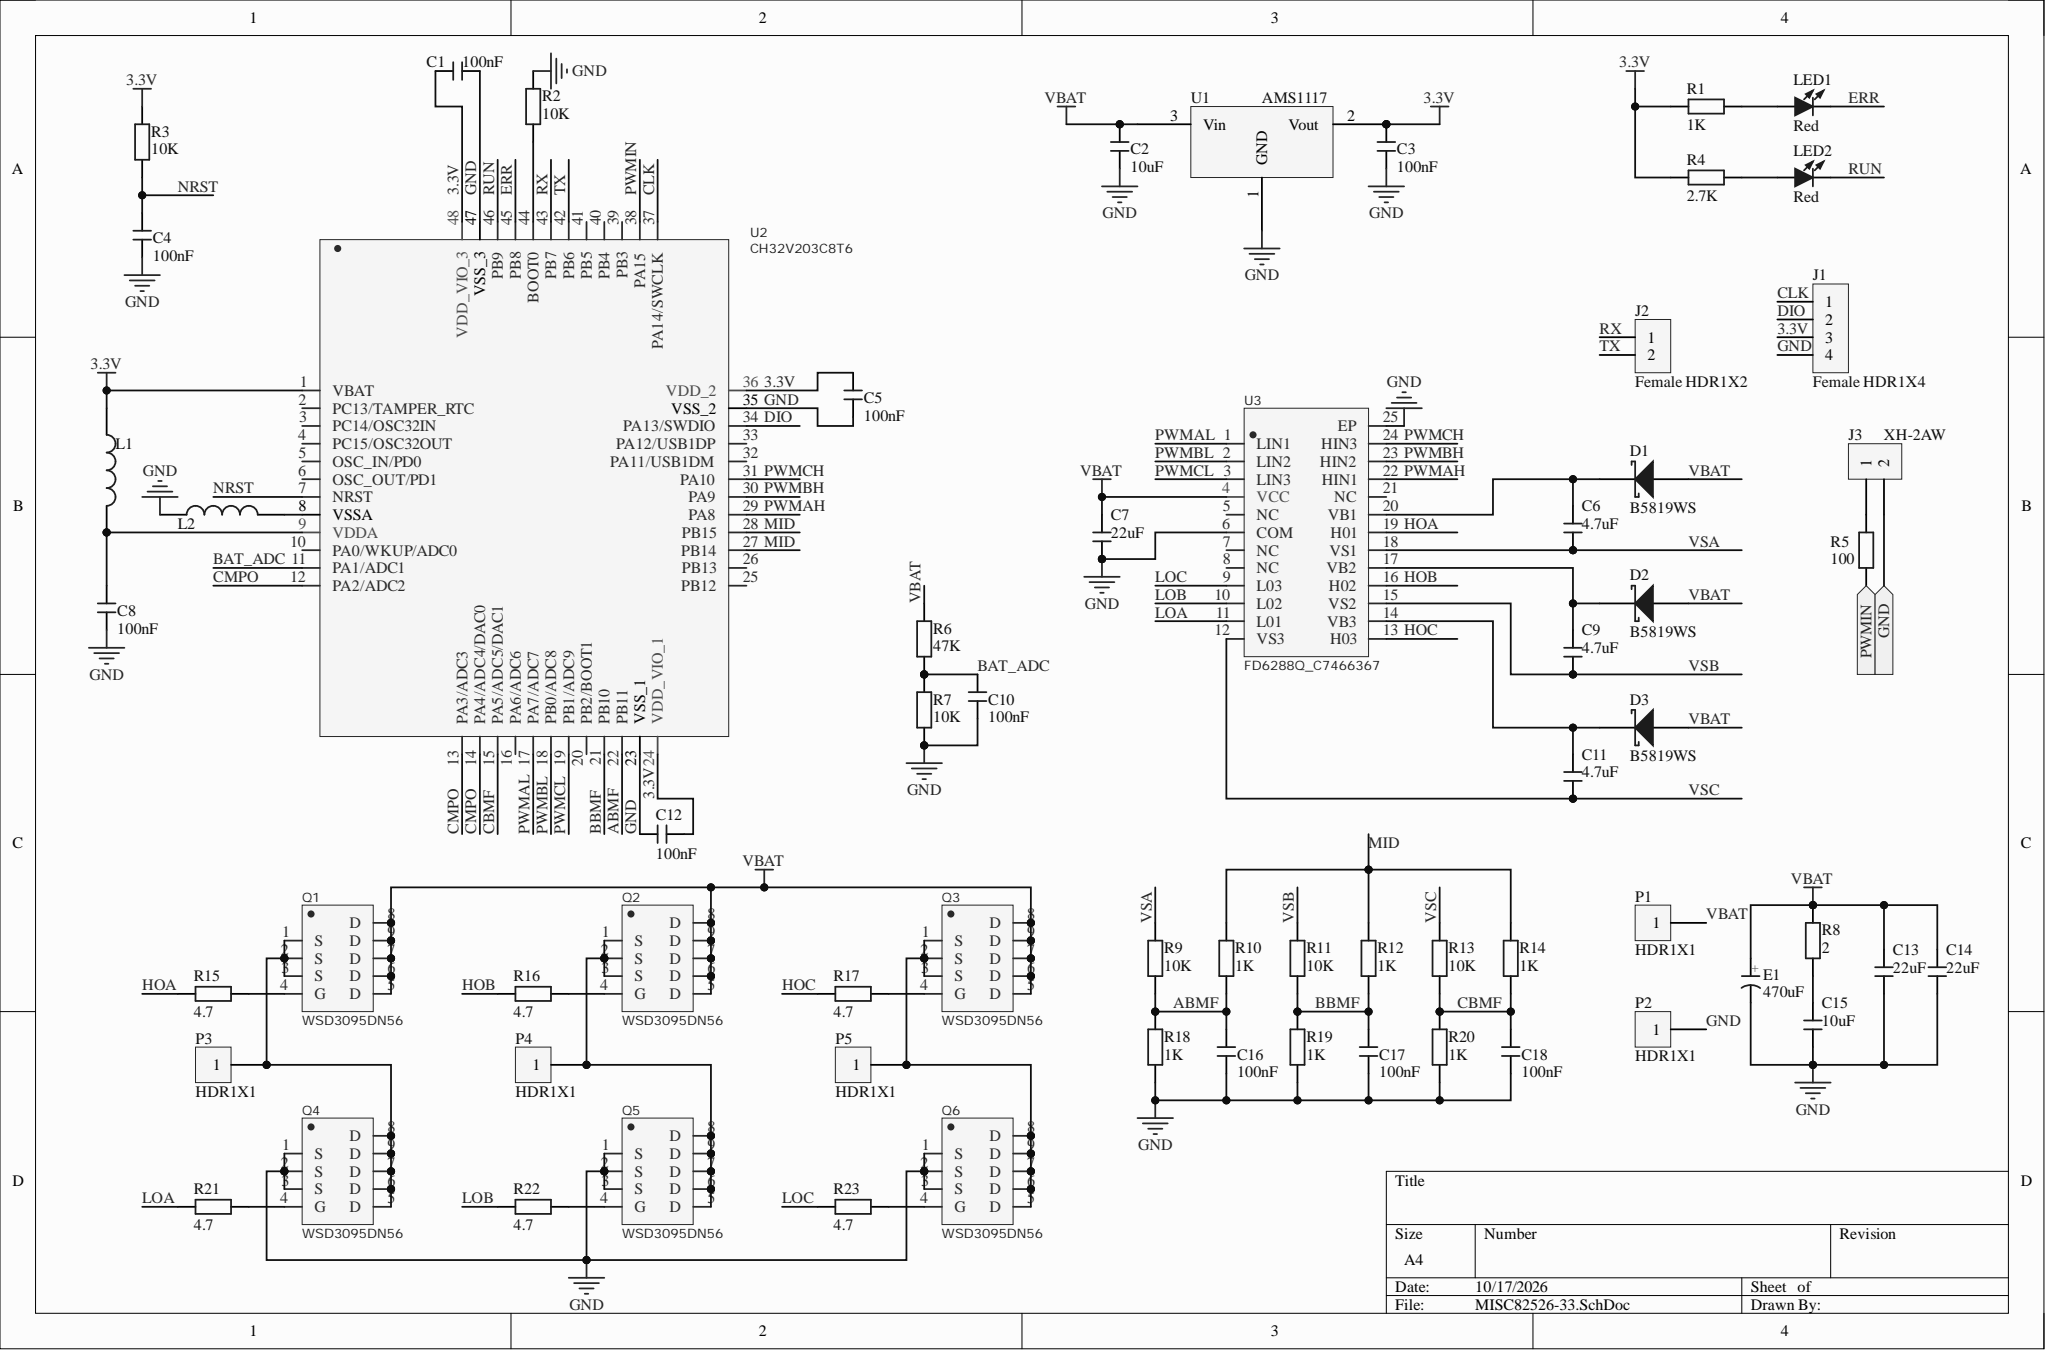Circuit board | Altium Designer | 66 parts | 50 nets
Bill of materials:
Comment,Description,Designator,Footprint,LibRef,Quantity
"100nF","SMD capacitor","C1, C3, C4, C5, C8, C10, C12, C16, C17, C18","C 0603_L","C","10"
"10uF","SMD capacitor","C2","C 0603_L","C","1"
"4.7uF","SMD capacitor","C6, C9, C11","C 0805_L","C","3"
"22uF","SMD capacitor","C7, C13, C14","C 0805_L","C","3"
"10uF","SMD capacitor","C15","C 0805_L","C","1"
"B5819WS","Schottky diode","D1, D2, D3","SOD-323","1N5819","3"
"470uF","SMD electrolytic capacitor","E1","CM A(3*5.4)","CE_SMD","1"
"Female HDR1X4","","J1","Fe-HDR1X4/2.54-S","Female HDR1X4","1"
"Female HDR1X2","","J2","Fe-HDR1X2/2.54-S","Female HDR1X2","1"
"XH-2AW","","J3","Fe-HDR1X2/2.54-S","Female HDR1X2","1"
"10uH","Low-power SMD inductor","L1, L2","L 0805","L","2"
"Red","SMD LED","LED1, LED2","LED 0805G","LED-SMD","2"
"HDR1X1","","P1, P2, P3, P4, P5","HDR1X1","HDR1X1","5"
"WSD3095DN56","","Q1, Q2, Q3, Q4, Q5, Q6","PDFN-8_L5.2-W5.9-P1.27-LS6.2-BL","WSD3095DN56","6"
"1K","SMD resistor","R1, R10, R12, R14, R18, R19, R20","R 0603_L","R","7"
"10K","SMD resistor","R2, R3, R7, R9, R11, R13","R 0603_L","R","6"
"2.7K","SMD resistor","R4","R 0603_L","R","1"
"100","SMD resistor","R5","R 0603_L","R","1"
"47K","SMD resistor","R6","R 0603_L","R","1"
"2","SMD resistor","R8","R 0603_L","R","1"
"4.7","SMD resistor","R15, R16, R17, R21, R22, R23","R 0603_L","R","6"
"AMS1117","Three-terminal voltage regulator","U1","SOT223","AMS1117","1"
"CH32V203C8T6","","U2","LQFP-48_L7.0-W7.0-P0.50-LS9.0-BL","CH32V203C8T6","1"
"FD6288Q_C7466367","","U3","QFN-24_L4.0-W4.0-P0.50-BL-EP2.7","FD6288Q_C7466367","1"
Netlist (Protel format):
[
C1
C 0603_L
100nF



]
[
C2
C 0603_L
10uF



]
[
C3
C 0603_L
100nF



]
[
C4
C 0603_L
100nF



]
[
C5
C 0603_L
100nF



]
[
C6
C 0805_L
4.7uF



]
[
C7
C 0805_L
22uF



]
[
C8
C 0603_L
100nF



]
[
C9
C 0805_L
4.7uF



]
[
C10
C 0603_L
100nF



]
[
C11
C 0805_L
4.7uF



]
[
C12
C 0603_L
100nF



]
[
C13
C 0805_L
22uF



]
[
C14
C 0805_L
22uF



]
[
C15
C 0805_L
10uF



]
[
C16
C 0603_L
100nF



]
[
C17
C 0603_L
100nF



]
[
C18
C 0603_L
100nF



]
[
D1
SOD-323
B5819WS



]
[
D2
SOD-323
B5819WS



]
[
D3
SOD-323
B5819WS



]
[
E1
CM A(3*5.4)
470uF



]
[
J1
Fe-HDR1X4/2.54-S
Female HDR1X4



]
[
J2
Fe-HDR1X2/2.54-S
Female HDR1X2



]
[
J3
Fe-HDR1X2/2.54-S
XH-2AW



]
[
L1
L 0805
10uH



]
[
L2
L 0805
10uH



]
[
LED1
LED 0805G
Red



]
[
LED2
LED 0805G
Red



]
[
P1
HDR1X1
HDR1X1



]
[
P2
HDR1X1
HDR1X1



]
[
P3
HDR1X1
HDR1X1



]
[
P4
HDR1X1
HDR1X1



]
[
P5
HDR1X1
HDR1X1



]
[
Q1
PDFN-8_L5.2-W5.9-P1.27-LS6.2-BL
WSD3095DN56



]
[
Q2
PDFN-8_L5.2-W5.9-P1.27-LS6.2-BL
WSD3095DN56



]
[
Q3
PDFN-8_L5.2-W5.9-P1.27-LS6.2-BL
WSD3095DN56



]
[
Q4
PDFN-8_L5.2-W5.9-P1.27-LS6.2-BL
WSD3095DN56



]
[
Q5
PDFN-8_L5.2-W5.9-P1.27-LS6.2-BL
WSD3095DN56



]
[
Q6
PDFN-8_L5.2-W5.9-P1.27-LS6.2-BL
WSD3095DN56



]
[
R1
R 0603_L
1K



]
[
R2
R 0603_L
10K



]
[
R3
R 0603_L
10K



]
[
R4
R 0603_L
2.7K



]
[
R5
R 0603_L
100



]
[
R6
R 0603_L
47K



]
[
R7
R 0603_L
10K



]
[
R8
R 0603_L
2



]
[
R9
R 0603_L
10K



]
[
R10
R 0603_L
1K



]
[
R11
R 0603_L
10K



]
[
R12
R 0603_L
1K



]
[
R13
R 0603_L
10K



]
[
R14
R 0603_L
1K



]
[
R15
R 0603_L
4.7



]
[
R16
R 0603_L
4.7



]
[
R17
R 0603_L
4.7



]
[
R18
R 0603_L
1K



]
[
R19
R 0603_L
1K



]
[
R20
R 0603_L
1K



]
[
R21
R 0603_L
4.7



]
[
R22
R 0603_L
4.7



]
[
R23
R 0603_L
4.7



]
[
U1
SOT223
AMS1117



]
[
U2
LQFP-48_L7.0-W7.0-P0.50-LS9.0-BL
CH32V203C8T6



]
[
U3
QFN-24_L4.0-W4.0-P0.50-BL-EP2.7
FD6288Q_C7466367



]
(
VSC
C11-1
R13-2
U3-12
)
(
VSB
C9-1
R11-2
U3-15
)
(
VSA
C6-1
R9-2
U3-18
)
(
VBAT
C2-2
C7-2
C13-2
C14-2
D1-1
D2-1
D3-1
E1-1
P1-1
Q1-5
Q1-6
Q1-7
Q1-8
Q1-9
Q2-5
Q2-6
Q2-7
Q2-8
Q2-9
Q3-5
Q3-6
Q3-7
Q3-8
Q3-9
R6-2
R8-2
U1-3
U3-4
)
(
TX
J2-2
U2-42
)
(
RX
J2-1
U2-43
)
(
RUN
LED2-2
U2-46
)
(
PWMCL
U2-19
U3-3
)
(
PWMCH
U2-31
U3-24
)
(
PWMBL
U2-18
U3-2
)
(
PWMBH
U2-30
U3-23
)
(
PWMAL
U2-17
U3-1
)
(
PWMAH
U2-29
U3-22
)
(
NRST
C4-2
R3-1
U2-7
)
(
NetR2_1
R2-1
U2-44
)
(
NetQ6_4
Q6-4
R23-1
)
(
NetQ5_4
Q5-4
R22-1
)
(
NetQ4_4
Q4-4
R21-1
)
(
NetQ3_4
Q3-4
R17-1
)
(
NetQ2_4
Q2-4
R16-1
)
(
NetQ1_4
Q1-4
R15-1
)
(
NetP5_1
P5-1
Q3-1
Q3-2
Q3-3
Q6-5
Q6-6
Q6-7
Q6-8
Q6-9
)
(
NetP4_1
P4-1
Q2-1
Q2-2
Q2-3
Q5-5
Q5-6
Q5-7
Q5-8
Q5-9
)
(
NetP3_1
P3-1
Q1-1
Q1-2
Q1-3
Q4-5
Q4-6
Q4-7
Q4-8
Q4-9
)
(
NetLED2_1
LED2-1
R4-1
)
(
NetLED1_1
LED1-1
R1-1
)
(
NetL2_2
L2-2
U2-8
)
(
NetJ3_1
J3-1
R5-1
)
(
NetC15_2
C15-2
R8-1
)
(
NetC11_2
C11-2
D3-2
U3-14
)
(
NetC9_2
C9-2
D2-2
U3-17
)
(
NetC8_2
C8-2
L1-2
U2-9
)
(
NetC6_2
C6-2
D1-2
U3-20
)
(
MID
R10-2
R12-2
R14-2
U2-27
U2-28
)
(
LOC
R23-2
U3-9
)
(
LOB
R22-2
U3-10
)
(
LOA
R21-2
U3-11
)
(
HOC
R17-2
U3-13
)
(
HOB
R16-2
U3-16
)
(
HOA
R15-2
U3-19
)
(
GND
C1-2
C2-1
C3-1
C4-1
C5-1
C7-1
C8-1
C10-1
C12-2
C13-1
C14-1
C15-1
C16-1
C17-1
C18-1
E1-2
J1-4
L2-1
P2-1
Q4-1
Q4-2
Q4-3
Q5-1
Q5-2
Q5-3
Q6-1
Q6-2
Q6-3
R2-2
R7-1
R18-1
R19-1
R20-1
U1-1
U2-23
U2-35
U2-47
U3-6
U3-25
)
(
ERR
LED1-2
U2-45
)
(
DIO
J1-2
U2-34
)
(
CMPO
U2-12
U2-13
U2-14
)
(
CLK
J1-1
U2-37
)
(
CBMF
C18-2
R13-1
R14-1
R20-2
U2-15
)
(
BBMF
C17-2
R11-1
R12-1
R19-2
U2-21
)
(
BAT_ADC
C10-2
R6-1
R7-2
U2-11
)
(
ABMF
C16-2
R9-1
R10-1
R18-2
U2-22
)
(
3.3V
C1-1
C3-2
C5-2
C12-1
J1-3
L1-1
R1-2
R3-2
R4-2
U1-2
U2-1
U2-24
U2-36
U2-48
)